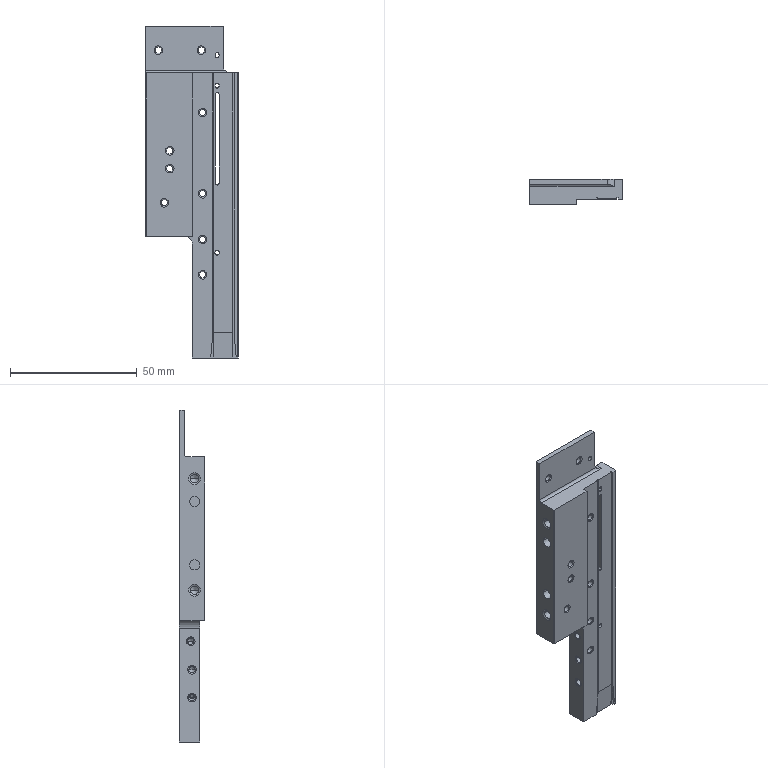Part | NX | 1 solid | 121 faces | box 36.55 x 10 x 131 mm | volume 27551 mm3 | cylinder 47 | cone 38 | plane 36 | commonest cylinder face diameters 2.5 x25 1.5 x9 3.3 x4 4 x4 1.8 x2 6 x2